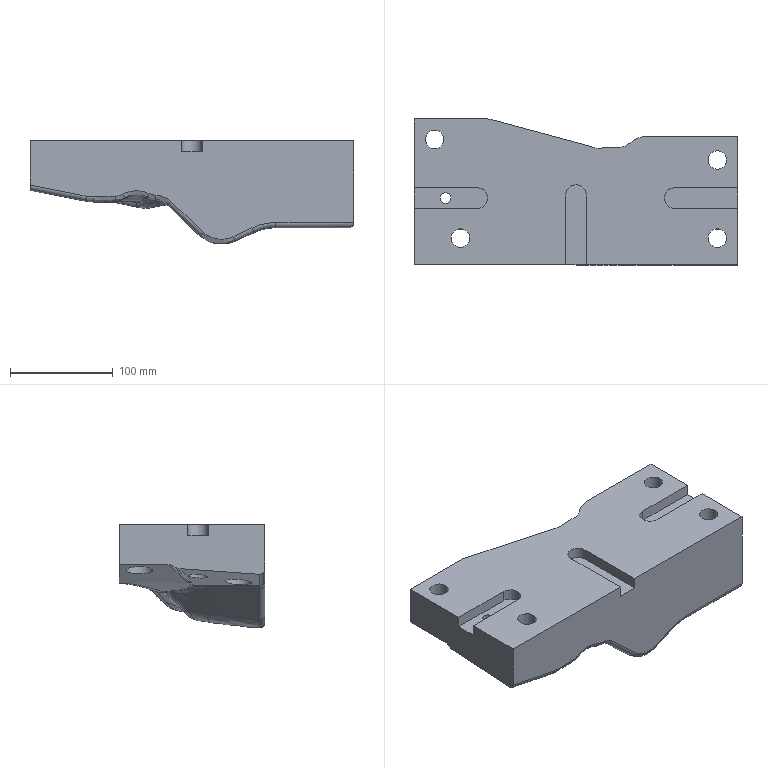Part | STEP file | lll_id582_x_t | 1 solid | 182 faces | box 315 x 142 x 100 mm | volume 2572181 mm3 | spline 101 | cylinder 37 | plane 35 | torus 4 | other 2 | cone 2 | sphere 1 | commonest cylinder face diameters 10 x7 20 x5 18.009 x4 26.008 x4 30 x4 40 x3